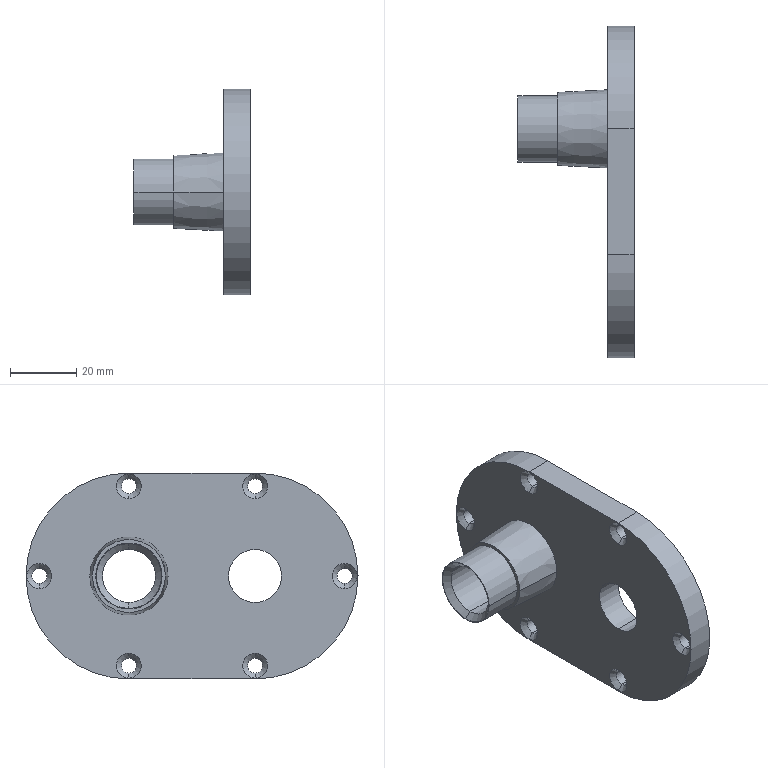Part | SolidWorks | features HoleWzd 3, Chamfer 1, Extrusion 1, Revolution 1 | 1 solid | 42 faces | box 35 x 100 x 62 mm | volume 43276 mm3 | cylinder 20 | cone 16 | plane 6 | commonest cylinder face diameters 4.5 x12 16 x4 20 x2 62 x2
STEP:
#1=CARTESIAN_POINT('',(1.5,-19.,24.75));
#2=VERTEX_POINT('',#1);
#3=CARTESIAN_POINT('',(1.5,-19.,29.25));
#4=VERTEX_POINT('',#3);
#5=CARTESIAN_POINT('',(1.5,-19.,27.));
#6=DIRECTION('',(-1.,0.,0.));
#7=DIRECTION('',(0.,0.,-1.));
#8=AXIS2_PLACEMENT_3D('',#5,#6,#7);
#9=CIRCLE('',#8,2.25);
#10=EDGE_CURVE('',#2,#4,#9,.T.);
#11=ORIENTED_EDGE('',*,*,#10,.F.);
#12=CARTESIAN_POINT('',(0.,-19.,23.25));
#13=VERTEX_POINT('',#12);
#14=CARTESIAN_POINT('',(1.5,-19.,24.75));
#15=DIRECTION('',(-0.7071,0.,-0.7071));
#16=VECTOR('',#15,1000.);
#17=LINE('',#14,#16);
#18=EDGE_CURVE('',#2,#13,#17,.T.);
#19=ORIENTED_EDGE('',*,*,#18,.T.);
#20=CARTESIAN_POINT('',(0.,-19.,30.75));
#21=VERTEX_POINT('',#20);
#22=CARTESIAN_POINT('',(0.,-19.,27.));
#23=DIRECTION('',(1.,0.,0.));
#24=DIRECTION('',(0.,0.,-1.));
#25=AXIS2_PLACEMENT_3D('',#22,#23,#24);
#26=CIRCLE('',#25,3.75);
#27=EDGE_CURVE('',#21,#13,#26,.T.);
#28=ORIENTED_EDGE('',*,*,#27,.F.);
#29=CARTESIAN_POINT('',(1.5,-19.,29.25));
#30=DIRECTION('',(-0.7071,0.,0.7071));
#31=VECTOR('',#30,1000.);
#32=LINE('',#29,#31);
#33=EDGE_CURVE('',#4,#21,#32,.T.);
#34=ORIENTED_EDGE('',*,*,#33,.F.);
#35=EDGE_LOOP('',(#11,#19,#28,#34));
#36=FACE_OUTER_BOUND('',#35,.T.);
#37=CARTESIAN_POINT('',(1.5,-19.,27.));
#38=DIRECTION('',(-1.,0.,0.));
#39=DIRECTION('',(0.,0.,1.));
#40=AXIS2_PLACEMENT_3D('',#37,#38,#39);
#41=CONICAL_SURFACE('',#40,2.25,0.7854);
#42=ADVANCED_FACE('',(#36),#41,.F.);
#43=CARTESIAN_POINT('',(1.5,-46.,-2.25));
#44=VERTEX_POINT('',#43);
#45=CARTESIAN_POINT('',(1.5,-46.,2.25));
#46=VERTEX_POINT('',#45);
#47=CARTESIAN_POINT('',(1.5,-46.,0.));
#48=DIRECTION('',(-1.,0.,0.));
#49=DIRECTION('',(0.,0.,-1.));
#50=AXIS2_PLACEMENT_3D('',#47,#48,#49);
#51=CIRCLE('',#50,2.25);
#52=EDGE_CURVE('',#44,#46,#51,.T.);
#53=ORIENTED_EDGE('',*,*,#52,.F.);
#54=CARTESIAN_POINT('',(0.,-46.,-3.75));
#55=VERTEX_POINT('',#54);
#56=CARTESIAN_POINT('',(1.5,-46.,-2.25));
#57=DIRECTION('',(-0.7071,0.,-0.7071));
#58=VECTOR('',#57,1000.);
#59=LINE('',#56,#58);
#60=EDGE_CURVE('',#44,#55,#59,.T.);
#61=ORIENTED_EDGE('',*,*,#60,.T.);
#62=CARTESIAN_POINT('',(0.,-46.,3.75));
#63=VERTEX_POINT('',#62);
#64=CARTESIAN_POINT('',(0.,-46.,0.));
#65=DIRECTION('',(1.,0.,0.));
#66=DIRECTION('',(0.,0.,-1.));
#67=AXIS2_PLACEMENT_3D('',#64,#65,#66);
#68=CIRCLE('',#67,3.75);
#69=EDGE_CURVE('',#63,#55,#68,.T.);
#70=ORIENTED_EDGE('',*,*,#69,.F.);
#71=CARTESIAN_POINT('',(1.5,-46.,2.25));
#72=DIRECTION('',(-0.7071,0.,0.7071));
#73=VECTOR('',#72,1000.);
#74=LINE('',#71,#73);
#75=EDGE_CURVE('',#46,#63,#74,.T.);
#76=ORIENTED_EDGE('',*,*,#75,.F.);
#77=EDGE_LOOP('',(#53,#61,#70,#76));
#78=FACE_OUTER_BOUND('',#77,.T.);
#79=CARTESIAN_POINT('',(1.5,-46.,0.));
#80=DIRECTION('',(-1.,0.,0.));
#81=DIRECTION('',(0.,0.,1.));
#82=AXIS2_PLACEMENT_3D('',#79,#80,#81);
#83=CONICAL_SURFACE('',#82,2.25,0.7854);
#84=ADVANCED_FACE('',(#78),#83,.F.);
#85=CARTESIAN_POINT('',(1.5,-19.,-29.25));
#86=VERTEX_POINT('',#85);
#87=CARTESIAN_POINT('',(1.5,-19.,-24.75));
#88=VERTEX_POINT('',#87);
#89=CARTESIAN_POINT('',(1.5,-19.,-27.));
#90=DIRECTION('',(-1.,0.,0.));
#91=DIRECTION('',(0.,0.,-1.));
#92=AXIS2_PLACEMENT_3D('',#89,#90,#91);
#93=CIRCLE('',#92,2.25);
#94=EDGE_CURVE('',#86,#88,#93,.T.);
#95=ORIENTED_EDGE('',*,*,#94,.F.);
#96=CARTESIAN_POINT('',(0.,-19.,-30.75));
#97=VERTEX_POINT('',#96);
#98=CARTESIAN_POINT('',(1.5,-19.,-29.25));
#99=DIRECTION('',(-0.7071,0.,-0.7071));
#100=VECTOR('',#99,1000.);
#101=LINE('',#98,#100);
#102=EDGE_CURVE('',#86,#97,#101,.T.);
#103=ORIENTED_EDGE('',*,*,#102,.T.);
#104=CARTESIAN_POINT('',(0.,-19.,-23.25));
#105=VERTEX_POINT('',#104);
#106=CARTESIAN_POINT('',(0.,-19.,-27.));
#107=DIRECTION('',(1.,0.,0.));
#108=DIRECTION('',(0.,0.,-1.));
#109=AXIS2_PLACEMENT_3D('',#106,#107,#108);
#110=CIRCLE('',#109,3.75);
#111=EDGE_CURVE('',#105,#97,#110,.T.);
#112=ORIENTED_EDGE('',*,*,#111,.F.);
#113=CARTESIAN_POINT('',(1.5,-19.,-24.75));
#114=DIRECTION('',(-0.7071,0.,0.7071));
#115=VECTOR('',#114,1000.);
#116=LINE('',#113,#115);
#117=EDGE_CURVE('',#88,#105,#116,.T.);
#118=ORIENTED_EDGE('',*,*,#117,.F.);
#119=EDGE_LOOP('',(#95,#103,#112,#118));
#120=FACE_OUTER_BOUND('',#119,.T.);
#121=CARTESIAN_POINT('',(1.5,-19.,-27.));
#122=DIRECTION('',(-1.,0.,0.));
#123=DIRECTION('',(0.,0.,1.));
#124=AXIS2_PLACEMENT_3D('',#121,#122,#123);
#125=CONICAL_SURFACE('',#124,2.25,0.7854);
#126=ADVANCED_FACE('',(#120),#125,.F.);
#127=CARTESIAN_POINT('',(1.5,19.,-29.25));
#128=VERTEX_POINT('',#127);
#129=CARTESIAN_POINT('',(1.5,19.,-24.75));
#130=VERTEX_POINT('',#129);
#131=CARTESIAN_POINT('',(1.5,19.,-27.));
#132=DIRECTION('',(-1.,0.,0.));
#133=DIRECTION('',(0.,0.,-1.));
#134=AXIS2_PLACEMENT_3D('',#131,#132,#133);
#135=CIRCLE('',#134,2.25);
#136=EDGE_CURVE('',#128,#130,#135,.T.);
#137=ORIENTED_EDGE('',*,*,#136,.F.);
#138=CARTESIAN_POINT('',(0.,19.,-30.75));
#139=VERTEX_POINT('',#138);
#140=CARTESIAN_POINT('',(1.5,19.,-29.25));
#141=DIRECTION('',(-0.7071,0.,-0.7071));
#142=VECTOR('',#141,1000.);
#143=LINE('',#140,#142);
#144=EDGE_CURVE('',#128,#139,#143,.T.);
#145=ORIENTED_EDGE('',*,*,#144,.T.);
#146=CARTESIAN_POINT('',(0.,19.,-23.25));
#147=VERTEX_POINT('',#146);
#148=CARTESIAN_POINT('',(0.,19.,-27.));
#149=DIRECTION('',(1.,0.,0.));
#150=DIRECTION('',(0.,0.,-1.));
#151=AXIS2_PLACEMENT_3D('',#148,#149,#150);
#152=CIRCLE('',#151,3.75);
#153=EDGE_CURVE('',#147,#139,#152,.T.);
#154=ORIENTED_EDGE('',*,*,#153,.F.);
#155=CARTESIAN_POINT('',(1.5,19.,-24.75));
#156=DIRECTION('',(-0.7071,0.,0.7071));
#157=VECTOR('',#156,1000.);
#158=LINE('',#155,#157);
#159=EDGE_CURVE('',#130,#147,#158,.T.);
#160=ORIENTED_EDGE('',*,*,#159,.F.);
#161=EDGE_LOOP('',(#137,#145,#154,#160));
#162=FACE_OUTER_BOUND('',#161,.T.);
#163=CARTESIAN_POINT('',(1.5,19.,-27.));
#164=DIRECTION('',(-1.,0.,0.));
#165=DIRECTION('',(0.,0.,1.));
#166=AXIS2_PLACEMENT_3D('',#163,#164,#165);
#167=CONICAL_SURFACE('',#166,2.25,0.7854);
#168=ADVANCED_FACE('',(#162),#167,.F.);
#169=CARTESIAN_POINT('',(1.5,46.,-2.25));
#170=VERTEX_POINT('',#169);
#171=CARTESIAN_POINT('',(1.5,46.,2.25));
#172=VERTEX_POINT('',#171);
#173=CARTESIAN_POINT('',(1.5,46.,0.));
#174=DIRECTION('',(-1.,0.,0.));
#175=DIRECTION('',(0.,0.,-1.));
#176=AXIS2_PLACEMENT_3D('',#173,#174,#175);
#177=CIRCLE('',#176,2.25);
#178=EDGE_CURVE('',#170,#172,#177,.T.);
#179=ORIENTED_EDGE('',*,*,#178,.F.);
#180=CARTESIAN_POINT('',(0.,46.,-3.75));
#181=VERTEX_POINT('',#180);
#182=CARTESIAN_POINT('',(1.5,46.,-2.25));
#183=DIRECTION('',(-0.7071,0.,-0.7071));
#184=VECTOR('',#183,1000.);
#185=LINE('',#182,#184);
#186=EDGE_CURVE('',#170,#181,#185,.T.);
#187=ORIENTED_EDGE('',*,*,#186,.T.);
#188=CARTESIAN_POINT('',(0.,46.,3.75));
#189=VERTEX_POINT('',#188);
#190=CARTESIAN_POINT('',(0.,46.,0.));
#191=DIRECTION('',(1.,0.,0.));
#192=DIRECTION('',(0.,0.,-1.));
#193=AXIS2_PLACEMENT_3D('',#190,#191,#192);
#194=CIRCLE('',#193,3.75);
#195=EDGE_CURVE('',#189,#181,#194,.T.);
#196=ORIENTED_EDGE('',*,*,#195,.F.);
#197=CARTESIAN_POINT('',(1.5,46.,2.25));
#198=DIRECTION('',(-0.7071,0.,0.7071));
#199=VECTOR('',#198,1000.);
#200=LINE('',#197,#199);
#201=EDGE_CURVE('',#172,#189,#200,.T.);
#202=ORIENTED_EDGE('',*,*,#201,.F.);
#203=EDGE_LOOP('',(#179,#187,#196,#202));
#204=FACE_OUTER_BOUND('',#203,.T.);
#205=CARTESIAN_POINT('',(1.5,46.,0.));
#206=DIRECTION('',(-1.,0.,0.));
#207=DIRECTION('',(0.,0.,1.));
#208=AXIS2_PLACEMENT_3D('',#205,#206,#207);
#209=CONICAL_SURFACE('',#208,2.25,0.7854);
#210=ADVANCED_FACE('',(#204),#209,.F.);
#211=CARTESIAN_POINT('',(1.5,19.,24.75));
#212=VERTEX_POINT('',#211);
#213=CARTESIAN_POINT('',(1.5,19.,29.25));
#214=VERTEX_POINT('',#213);
#215=CARTESIAN_POINT('',(1.5,19.,27.));
#216=DIRECTION('',(-1.,0.,0.));
#217=DIRECTION('',(0.,0.,-1.));
#218=AXIS2_PLACEMENT_3D('',#215,#216,#217);
#219=CIRCLE('',#218,2.25);
#220=EDGE_CURVE('',#212,#214,#219,.T.);
#221=ORIENTED_EDGE('',*,*,#220,.F.);
#222=CARTESIAN_POINT('',(0.,19.,23.25));
#223=VERTEX_POINT('',#222);
#224=CARTESIAN_POINT('',(1.5,19.,24.75));
#225=DIRECTION('',(-0.7071,0.,-0.7071));
#226=VECTOR('',#225,1000.);
#227=LINE('',#224,#226);
#228=EDGE_CURVE('',#212,#223,#227,.T.);
#229=ORIENTED_EDGE('',*,*,#228,.T.);
#230=CARTESIAN_POINT('',(0.,19.,30.75));
#231=VERTEX_POINT('',#230);
#232=CARTESIAN_POINT('',(0.,19.,27.));
#233=DIRECTION('',(1.,0.,0.));
#234=DIRECTION('',(0.,0.,-1.));
#235=AXIS2_PLACEMENT_3D('',#232,#233,#234);
#236=CIRCLE('',#235,3.75);
#237=EDGE_CURVE('',#231,#223,#236,.T.);
#238=ORIENTED_EDGE('',*,*,#237,.F.);
#239=CARTESIAN_POINT('',(1.5,19.,29.25));
#240=DIRECTION('',(-0.7071,0.,0.7071));
#241=VECTOR('',#240,1000.);
#242=LINE('',#239,#241);
#243=EDGE_CURVE('',#214,#231,#242,.T.);
#244=ORIENTED_EDGE('',*,*,#243,.F.);
#245=EDGE_LOOP('',(#221,#229,#238,#244));
#246=FACE_OUTER_BOUND('',#245,.T.);
#247=CARTESIAN_POINT('',(1.5,19.,27.));
#248=DIRECTION('',(-1.,0.,0.));
#249=DIRECTION('',(0.,0.,1.));
#250=AXIS2_PLACEMENT_3D('',#247,#248,#249);
#251=CONICAL_SURFACE('',#250,2.25,0.7854);
#252=ADVANCED_FACE('',(#246),#251,.F.);
#253=CARTESIAN_POINT('',(8.,46.,-2.25));
#254=VERTEX_POINT('',#253);
#255=CARTESIAN_POINT('',(8.,46.,2.25));
#256=VERTEX_POINT('',#255);
#257=CARTESIAN_POINT('',(8.,46.,0.));
#258=DIRECTION('',(-1.,0.,0.));
#259=DIRECTION('',(0.,0.,1.));
#260=AXIS2_PLACEMENT_3D('',#257,#258,#259);
#261=CIRCLE('',#260,2.25);
#262=EDGE_CURVE('',#254,#256,#261,.T.);
#263=ORIENTED_EDGE('',*,*,#262,.F.);
#264=CARTESIAN_POINT('',(0.,46.,-2.25));
#265=DIRECTION('',(-1.,0.,0.));
#266=VECTOR('',#265,1000.);
#267=LINE('',#264,#266);
#268=EDGE_CURVE('',#254,#170,#267,.T.);
#269=ORIENTED_EDGE('',*,*,#268,.T.);
#270=ORIENTED_EDGE('',*,*,#178,.T.);
#271=CARTESIAN_POINT('',(0.,46.,2.25));
#272=DIRECTION('',(-1.,0.,0.));
#273=VECTOR('',#272,1000.);
#274=LINE('',#271,#273);
#275=EDGE_CURVE('',#256,#172,#274,.T.);
#276=ORIENTED_EDGE('',*,*,#275,.F.);
#277=EDGE_LOOP('',(#263,#269,#270,#276));
#278=FACE_OUTER_BOUND('',#277,.T.);
#279=CARTESIAN_POINT('',(0.,46.,0.));
#280=DIRECTION('',(-1.,0.,0.));
#281=DIRECTION('',(0.,0.,1.));
#282=AXIS2_PLACEMENT_3D('',#279,#280,#281);
#283=CYLINDRICAL_SURFACE('',#282,2.25);
#284=ADVANCED_FACE('',(#278),#283,.F.);
#285=CARTESIAN_POINT('',(8.,19.,24.75));
#286=VERTEX_POINT('',#285);
#287=CARTESIAN_POINT('',(8.,19.,29.25));
#288=VERTEX_POINT('',#287);
#289=CARTESIAN_POINT('',(8.,19.,27.));
#290=DIRECTION('',(-1.,0.,0.));
#291=DIRECTION('',(0.,0.,1.));
#292=AXIS2_PLACEMENT_3D('',#289,#290,#291);
#293=CIRCLE('',#292,2.25);
#294=EDGE_CURVE('',#286,#288,#293,.T.);
#295=ORIENTED_EDGE('',*,*,#294,.F.);
#296=CARTESIAN_POINT('',(0.,19.,24.75));
#297=DIRECTION('',(-1.,0.,0.));
#298=VECTOR('',#297,1000.);
#299=LINE('',#296,#298);
#300=EDGE_CURVE('',#286,#212,#299,.T.);
#301=ORIENTED_EDGE('',*,*,#300,.T.);
#302=ORIENTED_EDGE('',*,*,#220,.T.);
#303=CARTESIAN_POINT('',(0.,19.,29.25));
#304=DIRECTION('',(-1.,0.,0.));
#305=VECTOR('',#304,1000.);
#306=LINE('',#303,#305);
#307=EDGE_CURVE('',#288,#214,#306,.T.);
#308=ORIENTED_EDGE('',*,*,#307,.F.);
#309=EDGE_LOOP('',(#295,#301,#302,#308));
#310=FACE_OUTER_BOUND('',#309,.T.);
#311=CARTESIAN_POINT('',(0.,19.,27.));
#312=DIRECTION('',(-1.,0.,0.));
#313=DIRECTION('',(0.,0.,1.));
#314=AXIS2_PLACEMENT_3D('',#311,#312,#313);
#315=CYLINDRICAL_SURFACE('',#314,2.25);
#316=ADVANCED_FACE('',(#310),#315,.F.);
#317=CARTESIAN_POINT('',(8.,19.,-29.25));
#318=VERTEX_POINT('',#317);
#319=CARTESIAN_POINT('',(8.,19.,-24.75));
#320=VERTEX_POINT('',#319);
#321=CARTESIAN_POINT('',(8.,19.,-27.));
#322=DIRECTION('',(-1.,0.,0.));
#323=DIRECTION('',(0.,0.,1.));
#324=AXIS2_PLACEMENT_3D('',#321,#322,#323);
#325=CIRCLE('',#324,2.25);
#326=EDGE_CURVE('',#318,#320,#325,.T.);
#327=ORIENTED_EDGE('',*,*,#326,.F.);
#328=CARTESIAN_POINT('',(0.,19.,-29.25));
#329=DIRECTION('',(-1.,0.,0.));
#330=VECTOR('',#329,1000.);
#331=LINE('',#328,#330);
#332=EDGE_CURVE('',#318,#128,#331,.T.);
#333=ORIENTED_EDGE('',*,*,#332,.T.);
#334=ORIENTED_EDGE('',*,*,#136,.T.);
#335=CARTESIAN_POINT('',(0.,19.,-24.75));
#336=DIRECTION('',(-1.,0.,0.));
#337=VECTOR('',#336,1000.);
#338=LINE('',#335,#337);
#339=EDGE_CURVE('',#320,#130,#338,.T.);
#340=ORIENTED_EDGE('',*,*,#339,.F.);
#341=EDGE_LOOP('',(#327,#333,#334,#340));
#342=FACE_OUTER_BOUND('',#341,.T.);
#343=CARTESIAN_POINT('',(0.,19.,-27.));
#344=DIRECTION('',(-1.,0.,0.));
#345=DIRECTION('',(0.,0.,1.));
#346=AXIS2_PLACEMENT_3D('',#343,#344,#345);
#347=CYLINDRICAL_SURFACE('',#346,2.25);
#348=ADVANCED_FACE('',(#342),#347,.F.);
#349=CARTESIAN_POINT('',(8.,-19.,24.75));
#350=VERTEX_POINT('',#349);
#351=CARTESIAN_POINT('',(8.,-19.,29.25));
#352=VERTEX_POINT('',#351);
#353=CARTESIAN_POINT('',(8.,-19.,27.));
#354=DIRECTION('',(-1.,0.,0.));
#355=DIRECTION('',(0.,0.,1.));
#356=AXIS2_PLACEMENT_3D('',#353,#354,#355);
#357=CIRCLE('',#356,2.25);
#358=EDGE_CURVE('',#350,#352,#357,.T.);
#359=ORIENTED_EDGE('',*,*,#358,.F.);
#360=CARTESIAN_POINT('',(0.,-19.,24.75));
#361=DIRECTION('',(-1.,0.,0.));
#362=VECTOR('',#361,1000.);
#363=LINE('',#360,#362);
#364=EDGE_CURVE('',#350,#2,#363,.T.);
#365=ORIENTED_EDGE('',*,*,#364,.T.);
#366=ORIENTED_EDGE('',*,*,#10,.T.);
#367=CARTESIAN_POINT('',(0.,-19.,29.25));
#368=DIRECTION('',(-1.,0.,0.));
#369=VECTOR('',#368,1000.);
#370=LINE('',#367,#369);
#371=EDGE_CURVE('',#352,#4,#370,.T.);
#372=ORIENTED_EDGE('',*,*,#371,.F.);
#373=EDGE_LOOP('',(#359,#365,#366,#372));
#374=FACE_OUTER_BOUND('',#373,.T.);
#375=CARTESIAN_POINT('',(0.,-19.,27.));
#376=DIRECTION('',(-1.,0.,0.));
#377=DIRECTION('',(0.,0.,1.));
#378=AXIS2_PLACEMENT_3D('',#375,#376,#377);
#379=CYLINDRICAL_SURFACE('',#378,2.25);
#380=ADVANCED_FACE('',(#374),#379,.F.);
#381=CARTESIAN_POINT('',(8.,-19.,-29.25));
#382=VERTEX_POINT('',#381);
#383=CARTESIAN_POINT('',(8.,-19.,-24.75));
#384=VERTEX_POINT('',#383);
#385=CARTESIAN_POINT('',(8.,-19.,-27.));
#386=DIRECTION('',(-1.,0.,0.));
#387=DIRECTION('',(0.,0.,1.));
#388=AXIS2_PLACEMENT_3D('',#385,#386,#387);
#389=CIRCLE('',#388,2.25);
#390=EDGE_CURVE('',#382,#384,#389,.T.);
#391=ORIENTED_EDGE('',*,*,#390,.F.);
#392=CARTESIAN_POINT('',(0.,-19.,-29.25));
#393=DIRECTION('',(-1.,0.,0.));
#394=VECTOR('',#393,1000.);
#395=LINE('',#392,#394);
#396=EDGE_CURVE('',#382,#86,#395,.T.);
#397=ORIENTED_EDGE('',*,*,#396,.T.);
#398=ORIENTED_EDGE('',*,*,#94,.T.);
#399=CARTESIAN_POINT('',(0.,-19.,-24.75));
#400=DIRECTION('',(-1.,0.,0.));
#401=VECTOR('',#400,1000.);
#402=LINE('',#399,#401);
#403=EDGE_CURVE('',#384,#88,#402,.T.);
#404=ORIENTED_EDGE('',*,*,#403,.F.);
#405=EDGE_LOOP('',(#391,#397,#398,#404));
#406=FACE_OUTER_BOUND('',#405,.T.);
#407=CARTESIAN_POINT('',(0.,-19.,-27.));
#408=DIRECTION('',(-1.,0.,0.));
#409=DIRECTION('',(0.,0.,1.));
#410=AXIS2_PLACEMENT_3D('',#407,#408,#409);
#411=CYLINDRICAL_SURFACE('',#410,2.25);
#412=ADVANCED_FACE('',(#406),#411,.F.);
#413=CARTESIAN_POINT('',(8.,-46.,-2.25));
#414=VERTEX_POINT('',#413);
#415=CARTESIAN_POINT('',(8.,-46.,2.25));
#416=VERTEX_POINT('',#415);
#417=CARTESIAN_POINT('',(8.,-46.,0.));
#418=DIRECTION('',(-1.,0.,0.));
#419=DIRECTION('',(0.,0.,1.));
#420=AXIS2_PLACEMENT_3D('',#417,#418,#419);
#421=CIRCLE('',#420,2.25);
#422=EDGE_CURVE('',#414,#416,#421,.T.);
#423=ORIENTED_EDGE('',*,*,#422,.F.);
#424=CARTESIAN_POINT('',(0.,-46.,-2.25));
#425=DIRECTION('',(-1.,0.,0.));
#426=VECTOR('',#425,1000.);
#427=LINE('',#424,#426);
#428=EDGE_CURVE('',#414,#44,#427,.T.);
#429=ORIENTED_EDGE('',*,*,#428,.T.);
#430=ORIENTED_EDGE('',*,*,#52,.T.);
#431=CARTESIAN_POINT('',(0.,-46.,2.25));
#432=DIRECTION('',(-1.,0.,0.));
#433=VECTOR('',#432,1000.);
#434=LINE('',#431,#433);
#435=EDGE_CURVE('',#416,#46,#434,.T.);
#436=ORIENTED_EDGE('',*,*,#435,.F.);
#437=EDGE_LOOP('',(#423,#429,#430,#436));
#438=FACE_OUTER_BOUND('',#437,.T.);
#439=CARTESIAN_POINT('',(0.,-46.,0.));
#440=DIRECTION('',(-1.,0.,0.));
#441=DIRECTION('',(0.,0.,1.));
#442=AXIS2_PLACEMENT_3D('',#439,#440,#441);
#443=CYLINDRICAL_SURFACE('',#442,2.25);
#444=ADVANCED_FACE('',(#438),#443,.F.);
#445=CARTESIAN_POINT('',(-25.2,19.,-8.));
#446=VERTEX_POINT('',#445);
#447=CARTESIAN_POINT('',(-25.2,19.,8.));
#448=VERTEX_POINT('',#447);
#449=CARTESIAN_POINT('',(-25.2,19.,0.));
#450=DIRECTION('',(-1.,0.,0.));
#451=DIRECTION('',(0.,0.,1.));
#452=AXIS2_PLACEMENT_3D('',#449,#450,#451);
#453=CIRCLE('',#452,8.);
#454=EDGE_CURVE('',#446,#448,#453,.T.);
#455=ORIENTED_EDGE('',*,*,#454,.F.);
#456=CARTESIAN_POINT('',(-27.,19.,-9.8));
#457=VERTEX_POINT('',#456);
#458=CARTESIAN_POINT('',(-27.,19.,-9.8));
#459=DIRECTION('',(-0.7071,0.,-0.7071));
#460=VECTOR('',#459,1000.);
#461=LINE('',#458,#460);
#462=EDGE_CURVE('',#446,#457,#461,.T.);
#463=ORIENTED_EDGE('',*,*,#462,.T.);
#464=CARTESIAN_POINT('',(-27.,19.,9.8));
#465=VERTEX_POINT('',#464);
#466=CARTESIAN_POINT('',(-27.,19.,0.));
#467=DIRECTION('',(-1.,0.,0.));
#468=DIRECTION('',(0.,0.,1.));
#469=AXIS2_PLACEMENT_3D('',#466,#467,#468);
#470=CIRCLE('',#469,9.8);
#471=EDGE_CURVE('',#457,#465,#470,.T.);
#472=ORIENTED_EDGE('',*,*,#471,.T.);
#473=CARTESIAN_POINT('',(-27.,19.,9.8));
#474=DIRECTION('',(-0.7071,0.,0.7071));
#475=VECTOR('',#474,1000.);
#476=LINE('',#473,#475);
#477=EDGE_CURVE('',#448,#465,#476,.T.);
#478=ORIENTED_EDGE('',*,*,#477,.F.);
#479=EDGE_LOOP('',(#455,#463,#472,#478));
#480=FACE_OUTER_BOUND('',#479,.T.);
#481=CARTESIAN_POINT('',(-27.,19.,0.));
#482=DIRECTION('',(-1.,0.,0.));
#483=DIRECTION('',(0.,0.,1.));
#484=AXIS2_PLACEMENT_3D('',#481,#482,#483);
#485=CONICAL_SURFACE('',#484,9.8,0.7854);
#486=ADVANCED_FACE('',(#480),#485,.F.);
#487=CARTESIAN_POINT('',(8.,19.,-8.));
#488=VERTEX_POINT('',#487);
#489=CARTESIAN_POINT('',(8.,19.,8.));
#490=VERTEX_POINT('',#489);
#491=CARTESIAN_POINT('',(8.,19.,0.));
#492=DIRECTION('',(-1.,0.,0.));
#493=DIRECTION('',(0.,0.,1.));
#494=AXIS2_PLACEMENT_3D('',#491,#492,#493);
#495=CIRCLE('',#494,8.);
#496=EDGE_CURVE('',#488,#490,#495,.T.);
#497=ORIENTED_EDGE('',*,*,#496,.F.);
#498=CARTESIAN_POINT('',(-27.,19.,-8.));
#499=DIRECTION('',(-1.,0.,0.));
#500=VECTOR('',#499,1000.);
#501=LINE('',#498,#500);
#502=EDGE_CURVE('',#488,#446,#501,.T.);
#503=ORIENTED_EDGE('',*,*,#502,.T.);
#504=ORIENTED_EDGE('',*,*,#454,.T.);
#505=CARTESIAN_POINT('',(-27.,19.,8.));
#506=DIRECTION('',(-1.,0.,0.));
#507=VECTOR('',#506,1000.);
#508=LINE('',#505,#507);
#509=EDGE_CURVE('',#490,#448,#508,.T.);
#510=ORIENTED_EDGE('',*,*,#509,.F.);
#511=EDGE_LOOP('',(#497,#503,#504,#510));
#512=FACE_OUTER_BOUND('',#511,.T.);
#513=CARTESIAN_POINT('',(-27.,19.,0.));
#514=DIRECTION('',(-1.,0.,0.));
#515=DIRECTION('',(0.,0.,1.));
#516=AXIS2_PLACEMENT_3D('',#513,#514,#515);
#517=CYLINDRICAL_SURFACE('',#516,8.);
#518=ADVANCED_FACE('',(#512),#517,.F.);
#519=CARTESIAN_POINT('',(8.,-19.,-8.));
#520=VERTEX_POINT('',#519);
#521=CARTESIAN_POINT('',(8.,-19.,8.));
#522=VERTEX_POINT('',#521);
#523=CARTESIAN_POINT('',(8.,-19.,0.));
#524=DIRECTION('',(-1.,0.,0.));
#525=DIRECTION('',(0.,0.,1.));
#526=AXIS2_PLACEMENT_3D('',#523,#524,#525);
#527=CIRCLE('',#526,8.);
#528=EDGE_CURVE('',#520,#522,#527,.T.);
#529=ORIENTED_EDGE('',*,*,#528,.F.);
#530=CARTESIAN_POINT('',(0.,-19.,-8.));
#531=VERTEX_POINT('',#530);
#532=CARTESIAN_POINT('',(0.,-19.,-8.));
#533=DIRECTION('',(-1.,0.,0.));
#534=VECTOR('',#533,1000.);
#535=LINE('',#532,#534);
#536=EDGE_CURVE('',#520,#531,#535,.T.);
#537=ORIENTED_EDGE('',*,*,#536,.T.);
#538=CARTESIAN_POINT('',(0.,-19.,8.));
#539=VERTEX_POINT('',#538);
#540=CARTESIAN_POINT('',(0.,-19.,0.));
#541=DIRECTION('',(-1.,0.,0.));
#542=DIRECTION('',(0.,0.,1.));
#543=AXIS2_PLACEMENT_3D('',#540,#541,#542);
#544=CIRCLE('',#543,8.);
#545=EDGE_CURVE('',#531,#539,#544,.T.);
#546=ORIENTED_EDGE('',*,*,#545,.T.);
#547=CARTESIAN_POINT('',(0.,-19.,8.));
#548=DIRECTION('',(-1.,0.,0.));
#549=VECTOR('',#548,1000.);
#550=LINE('',#547,#549);
#551=EDGE_CURVE('',#522,#539,#550,.T.);
#552=ORIENTED_EDGE('',*,*,#551,.F.);
#553=EDGE_LOOP('',(#529,#537,#546,#552));
#554=FACE_OUTER_BOUND('',#553,.T.);
#555=CARTESIAN_POINT('',(0.,-19.,0.));
#556=DIRECTION('',(-1.,0.,0.));
#557=DIRECTION('',(0.,0.,1.));
#558=AXIS2_PLACEMENT_3D('',#555,#556,#557);
#559=CYLINDRICAL_SURFACE('',#558,8.);
#560=ADVANCED_FACE('',(#554),#559,.F.);
#561=CARTESIAN_POINT('',(-15.,30.,0.));
#562=VERTEX_POINT('',#561);
#563=CARTESIAN_POINT('',(-15.,8.,0.));
#564=VERTEX_POINT('',#563);
#565=CARTESIAN_POINT('',(-15.,19.,0.));
#566=DIRECTION('',(1.,0.,0.));
#567=DIRECTION('',(0.,1.,0.));
#568=AXIS2_PLACEMENT_3D('',#565,#566,#567);
#569=CIRCLE('',#568,11.);
#570=EDGE_CURVE('',#562,#564,#569,.T.);
#571=ORIENTED_EDGE('',*,*,#570,.T.);
#572=CARTESIAN_POINT('',(0.,7.214,0.));
#573=VERTEX_POINT('',#572);
#574=CARTESIAN_POINT('',(0.,7.214,0.));
#575=DIRECTION('',(0.9986,-0.05234,0.));
#576=VECTOR('',#575,1000.);
#577=LINE('',#574,#576);
#578=EDGE_CURVE('',#564,#573,#577,.T.);
#579=ORIENTED_EDGE('',*,*,#578,.T.);
#580=CARTESIAN_POINT('',(0.,30.786,0.));
#581=VERTEX_POINT('',#580);
#582=CARTESIAN_POINT('',(0.,19.,0.));
#583=DIRECTION('',(1.,0.,0.));
#584=DIRECTION('',(0.,1.,0.));
#585=AXIS2_PLACEMENT_3D('',#582,#583,#584);
#586=CIRCLE('',#585,11.786);
#587=EDGE_CURVE('',#581,#573,#586,.T.);
#588=ORIENTED_EDGE('',*,*,#587,.F.);
#589=CARTESIAN_POINT('',(0.,30.786,0.));
#590=DIRECTION('',(0.9986,0.05234,0.));
#591=VECTOR('',#590,1000.);
#592=LINE('',#589,#591);
#593=EDGE_CURVE('',#562,#581,#592,.T.);
#594=ORIENTED_EDGE('',*,*,#593,.F.);
#595=EDGE_LOOP('',(#571,#579,#588,#594));
#596=FACE_OUTER_BOUND('',#595,.T.);
#597=CARTESIAN_POINT('',(0.,19.,0.));
#598=DIRECTION('',(1.,0.,0.));
#599=DIRECTION('',(0.,1.,0.));
#600=AXIS2_PLACEMENT_3D('',#597,#598,#599);
#601=CONICAL_SURFACE('',#600,11.786,0.05236);
#602=ADVANCED_FACE('',(#596),#601,.T.);
#603=CARTESIAN_POINT('',(-27.,29.,0.));
#604=VERTEX_POINT('',#603);
#605=CARTESIAN_POINT('',(-27.,9.,0.));
#606=VERTEX_POINT('',#605);
#607=CARTESIAN_POINT('',(-27.,19.,0.));
#608=DIRECTION('',(1.,0.,0.));
#609=DIRECTION('',(0.,1.,0.));
#610=AXIS2_PLACEMENT_3D('',#607,#608,#609);
#611=CIRCLE('',#610,10.);
#612=EDGE_CURVE('',#604,#606,#611,.T.);
#613=ORIENTED_EDGE('',*,*,#612,.T.);
#614=CARTESIAN_POINT('',(-15.,9.,0.));
#615=VERTEX_POINT('',#614);
#616=CARTESIAN_POINT('',(-27.,9.,0.));
#617=DIRECTION('',(1.,0.,0.));
#618=VECTOR('',#617,1000.);
#619=LINE('',#616,#618);
#620=EDGE_CURVE('',#606,#615,#619,.T.);
#621=ORIENTED_EDGE('',*,*,#620,.T.);
#622=CARTESIAN_POINT('',(-15.,29.,0.));
#623=VERTEX_POINT('',#622);
#624=CARTESIAN_POINT('',(-15.,19.,0.));
#625=DIRECTION('',(1.,0.,0.));
#626=DIRECTION('',(0.,1.,0.));
#627=AXIS2_PLACEMENT_3D('',#624,#625,#626);
#628=CIRCLE('',#627,10.);
#629=EDGE_CURVE('',#623,#615,#628,.T.);
#630=ORIENTED_EDGE('',*,*,#629,.F.);
#631=CARTESIAN_POINT('',(-27.,29.,0.));
#632=DIRECTION('',(1.,0.,0.));
#633=VECTOR('',#632,1000.);
#634=LINE('',#631,#633);
#635=EDGE_CURVE('',#604,#623,#634,.T.);
#636=ORIENTED_EDGE('',*,*,#635,.F.);
#637=EDGE_LOOP('',(#613,#621,#630,#636));
#638=FACE_OUTER_BOUND('',#637,.T.);
#639=CARTESIAN_POINT('',(-27.,19.,0.));
#640=DIRECTION('',(1.,0.,0.));
#641=DIRECTION('',(0.,1.,0.));
#642=AXIS2_PLACEMENT_3D('',#639,#640,#641);
#643=CYLINDRICAL_SURFACE('',#642,10.);
#644=ADVANCED_FACE('',(#638),#643,.T.);
#645=CARTESIAN_POINT('',(8.,-19.,31.));
#646=VERTEX_POINT('',#645);
#647=CARTESIAN_POINT('',(8.,-19.,-31.));
#648=VERTEX_POINT('',#647);
#649=CARTESIAN_POINT('',(8.,-19.,0.));
#650=DIRECTION('',(1.,0.,0.));
#651=DIRECTION('',(0.,0.,-1.));
#652=AXIS2_PLACEMENT_3D('',#649,#650,#651);
#653=CIRCLE('',#652,31.);
#654=EDGE_CURVE('',#646,#648,#653,.T.);
#655=ORIENTED_EDGE('',*,*,#654,.F.);
#656=CARTESIAN_POINT('',(0.,-19.,31.));
#657=VERTEX_POINT('',#656);
#658=CARTESIAN_POINT('',(0.,-19.,31.));
#659=DIRECTION('',(1.,0.,0.));
#660=VECTOR('',#659,1000.);
#661=LINE('',#658,#660);
#662=EDGE_CURVE('',#657,#646,#661,.T.);
#663=ORIENTED_EDGE('',*,*,#662,.F.);
#664=CARTESIAN_POINT('',(0.,-19.,-31.));
#665=VERTEX_POINT('',#664);
#666=CARTESIAN_POINT('',(0.,-19.,0.));
#667=DIRECTION('',(1.,0.,0.));
#668=DIRECTION('',(0.,0.,-1.));
#669=AXIS2_PLACEMENT_3D('',#666,#667,#668);
#670=CIRCLE('',#669,31.);
#671=EDGE_CURVE('',#657,#665,#670,.T.);
#672=ORIENTED_EDGE('',*,*,#671,.T.);
#673=CARTESIAN_POINT('',(0.,-19.,-31.));
#674=DIRECTION('',(1.,0.,0.));
#675=VECTOR('',#674,1000.);
#676=LINE('',#673,#675);
#677=EDGE_CURVE('',#665,#648,#676,.T.);
#678=ORIENTED_EDGE('',*,*,#677,.T.);
#679=EDGE_LOOP('',(#655,#663,#672,#678));
#680=FACE_OUTER_BOUND('',#679,.T.);
#681=CARTESIAN_POINT('',(0.,-19.,0.));
#682=DIRECTION('',(1.,0.,0.));
#683=DIRECTION('',(0.,0.,-1.));
#684=AXIS2_PLACEMENT_3D('',#681,#682,#683);
#685=CYLINDRICAL_SURFACE('',#684,31.);
#686=ADVANCED_FACE('',(#680),#685,.T.);
#687=CARTESIAN_POINT('',(8.,19.,31.));
#688=VERTEX_POINT('',#687);
#689=CARTESIAN_POINT('',(8.,19.,31.));
#690=DIRECTION('',(0.,-1.,0.));
#691=VECTOR('',#690,1000.);
#692=LINE('',#689,#691);
#693=EDGE_CURVE('',#688,#646,#692,.T.);
#694=ORIENTED_EDGE('',*,*,#693,.F.);
#695=CARTESIAN_POINT('',(0.,19.,31.));
#696=VERTEX_POINT('',#695);
#697=CARTESIAN_POINT('',(0.,19.,31.));
#698=DIRECTION('',(1.,0.,0.));
#699=VECTOR('',#698,1000.);
#700=LINE('',#697,#699);
#701=EDGE_CURVE('',#696,#688,#700,.T.);
#702=ORIENTED_EDGE('',*,*,#701,.F.);
#703=CARTESIAN_POINT('',(0.,19.,31.));
#704=DIRECTION('',(0.,-1.,0.));
#705=VECTOR('',#704,1000.);
#706=LINE('',#703,#705);
#707=EDGE_CURVE('',#696,#657,#706,.T.);
#708=ORIENTED_EDGE('',*,*,#707,.T.);
#709=ORIENTED_EDGE('',*,*,#662,.T.);
#710=EDGE_LOOP('',(#694,#702,#708,#709));
#711=FACE_OUTER_BOUND('',#710,.T.);
#712=CARTESIAN_POINT('',(0.,19.,31.));
#713=DIRECTION('',(0.,0.,1.));
#714=DIRECTION('',(1.,0.,0.));
#715=AXIS2_PLACEMENT_3D('',#712,#713,#714);
#716=PLANE('',#715);
#717=ADVANCED_FACE('',(#711),#716,.T.);
#718=CARTESIAN_POINT('',(8.,19.,-31.));
#719=VERTEX_POINT('',#718);
#720=CARTESIAN_POINT('',(8.,19.,0.));
#721=DIRECTION('',(1.,0.,0.));
#722=DIRECTION('',(0.,0.,-1.));
#723=AXIS2_PLACEMENT_3D('',#720,#721,#722);
#724=CIRCLE('',#723,31.);
#725=EDGE_CURVE('',#719,#688,#724,.T.);
#726=ORIENTED_EDGE('',*,*,#725,.F.);
#727=CARTESIAN_POINT('',(0.,19.,-31.));
#728=VERTEX_POINT('',#727);
#729=CARTESIAN_POINT('',(0.,19.,-31.));
#730=DIRECTION('',(1.,0.,0.));
#731=VECTOR('',#730,1000.);
#732=LINE('',#729,#731);
#733=EDGE_CURVE('',#728,#719,#732,.T.);
#734=ORIENTED_EDGE('',*,*,#733,.F.);
#735=CARTESIAN_POINT('',(0.,19.,0.));
#736=DIRECTION('',(1.,0.,0.));
#737=DIRECTION('',(0.,0.,-1.));
#738=AXIS2_PLACEMENT_3D('',#735,#736,#737);
#739=CIRCLE('',#738,31.);
#740=EDGE_CURVE('',#728,#696,#739,.T.);
#741=ORIENTED_EDGE('',*,*,#740,.T.);
#742=ORIENTED_EDGE('',*,*,#701,.T.);
#743=EDGE_LOOP('',(#726,#734,#741,#742));
#744=FACE_OUTER_BOUND('',#743,.T.);
#745=CARTESIAN_POINT('',(0.,19.,0.));
#746=DIRECTION('',(1.,0.,0.));
#747=DIRECTION('',(0.,0.,-1.));
#748=AXIS2_PLACEMENT_3D('',#745,#746,#747);
#749=CYLINDRICAL_SURFACE('',#748,31.);
#750=ADVANCED_FACE('',(#744),#749,.T.);
#751=CARTESIAN_POINT('',(8.,-19.,-31.));
#752=DIRECTION('',(0.,1.,0.));
#753=VECTOR('',#752,1000.);
#754=LINE('',#751,#753);
#755=EDGE_CURVE('',#648,#719,#754,.T.);
#756=ORIENTED_EDGE('',*,*,#755,.F.);
#757=ORIENTED_EDGE('',*,*,#677,.F.);
#758=CARTESIAN_POINT('',(0.,-19.,-31.));
#759=DIRECTION('',(0.,1.,0.));
#760=VECTOR('',#759,1000.);
#761=LINE('',#758,#760);
#762=EDGE_CURVE('',#665,#728,#761,.T.);
#763=ORIENTED_EDGE('',*,*,#762,.T.);
#764=ORIENTED_EDGE('',*,*,#733,.T.);
#765=EDGE_LOOP('',(#756,#757,#763,#764));
#766=FACE_OUTER_BOUND('',#765,.T.);
#767=CARTESIAN_POINT('',(0.,-19.,-31.));
#768=DIRECTION('',(0.,0.,-1.));
#769=DIRECTION('',(-1.,0.,0.));
#770=AXIS2_PLACEMENT_3D('',#767,#768,#769);
#771=PLANE('',#770);
#772=ADVANCED_FACE('',(#766),#771,.T.);
#773=ORIENTED_EDGE('',*,*,#237,.T.);
#774=CARTESIAN_POINT('',(0.,19.,27.));
#775=DIRECTION('',(1.,0.,0.));
#776=DIRECTION('',(0.,0.,-1.));
#777=AXIS2_PLACEMENT_3D('',#774,#775,#776);
#778=CIRCLE('',#777,3.75);
#779=EDGE_CURVE('',#223,#231,#778,.T.);
#780=ORIENTED_EDGE('',*,*,#779,.T.);
#781=EDGE_LOOP('',(#773,#780));
#782=FACE_BOUND('',#781,.T.);
#783=ORIENTED_EDGE('',*,*,#195,.T.);
#784=CARTESIAN_POINT('',(0.,46.,0.));
#785=DIRECTION('',(1.,0.,0.));
#786=DIRECTION('',(0.,0.,-1.));
#787=AXIS2_PLACEMENT_3D('',#784,#785,#786);
#788=CIRCLE('',#787,3.75);
#789=EDGE_CURVE('',#181,#189,#788,.T.);
#790=ORIENTED_EDGE('',*,*,#789,.T.);
#791=EDGE_LOOP('',(#783,#790));
#792=FACE_BOUND('',#791,.T.);
#793=ORIENTED_EDGE('',*,*,#153,.T.);
#794=CARTESIAN_POINT('',(0.,19.,-27.));
#795=DIRECTION('',(1.,0.,0.));
#796=DIRECTION('',(0.,0.,-1.));
#797=AXIS2_PLACEMENT_3D('',#794,#795,#796);
#798=CIRCLE('',#797,3.75);
#799=EDGE_CURVE('',#139,#147,#798,.T.);
#800=ORIENTED_EDGE('',*,*,#799,.T.);
#801=EDGE_LOOP('',(#793,#800));
#802=FACE_BOUND('',#801,.T.);
#803=ORIENTED_EDGE('',*,*,#111,.T.);
#804=CARTESIAN_POINT('',(0.,-19.,-27.));
#805=DIRECTION('',(1.,0.,0.));
#806=DIRECTION('',(0.,0.,-1.));
#807=AXIS2_PLACEMENT_3D('',#804,#805,#806);
#808=CIRCLE('',#807,3.75);
#809=EDGE_CURVE('',#97,#105,#808,.T.);
#810=ORIENTED_EDGE('',*,*,#809,.T.);
#811=EDGE_LOOP('',(#803,#810));
#812=FACE_BOUND('',#811,.T.);
#813=ORIENTED_EDGE('',*,*,#69,.T.);
#814=CARTESIAN_POINT('',(0.,-46.,0.));
#815=DIRECTION('',(1.,0.,0.));
#816=DIRECTION('',(0.,0.,-1.));
#817=AXIS2_PLACEMENT_3D('',#814,#815,#816);
#818=CIRCLE('',#817,3.75);
#819=EDGE_CURVE('',#55,#63,#818,.T.);
#820=ORIENTED_EDGE('',*,*,#819,.T.);
#821=EDGE_LOOP('',(#813,#820));
#822=FACE_BOUND('',#821,.T.);
#823=ORIENTED_EDGE('',*,*,#27,.T.);
#824=CARTESIAN_POINT('',(0.,-19.,27.));
#825=DIRECTION('',(1.,0.,0.));
#826=DIRECTION('',(0.,0.,-1.));
#827=AXIS2_PLACEMENT_3D('',#824,#825,#826);
#828=CIRCLE('',#827,3.75);
#829=EDGE_CURVE('',#13,#21,#828,.T.);
#830=ORIENTED_EDGE('',*,*,#829,.T.);
#831=EDGE_LOOP('',(#823,#830));
#832=FACE_BOUND('',#831,.T.);
#833=CARTESIAN_POINT('',(0.,-19.,0.));
#834=DIRECTION('',(-1.,0.,0.));
#835=DIRECTION('',(0.,0.,1.));
#836=AXIS2_PLACEMENT_3D('',#833,#834,#835);
#837=CIRCLE('',#836,8.);
#838=EDGE_CURVE('',#539,#531,#837,.T.);
#839=ORIENTED_EDGE('',*,*,#838,.F.);
#840=ORIENTED_EDGE('',*,*,#545,.F.);
#841=EDGE_LOOP('',(#839,#840));
#842=FACE_BOUND('',#841,.T.);
#843=ORIENTED_EDGE('',*,*,#587,.T.);
#844=CARTESIAN_POINT('',(0.,19.,0.));
#845=DIRECTION('',(1.,0.,0.));
#846=DIRECTION('',(0.,1.,0.));
#847=AXIS2_PLACEMENT_3D('',#844,#845,#846);
#848=CIRCLE('',#847,11.786);
#849=EDGE_CURVE('',#573,#581,#848,.T.);
#850=ORIENTED_EDGE('',*,*,#849,.T.);
#851=EDGE_LOOP('',(#843,#850));
#852=FACE_BOUND('',#851,.T.);
#853=ORIENTED_EDGE('',*,*,#671,.F.);
#854=ORIENTED_EDGE('',*,*,#707,.F.);
#855=ORIENTED_EDGE('',*,*,#740,.F.);
#856=ORIENTED_EDGE('',*,*,#762,.F.);
#857=EDGE_LOOP('',(#853,#854,#855,#856));
#858=FACE_OUTER_BOUND('',#857,.T.);
#859=CARTESIAN_POINT('',(0.,-19.,0.));
#860=DIRECTION('',(1.,0.,0.));
#861=DIRECTION('',(0.,0.,-1.));
#862=AXIS2_PLACEMENT_3D('',#859,#860,#861);
#863=PLANE('',#862);
#864=ADVANCED_FACE('',(#782,#792,#802,#812,#822,#832,#842,#852,#858),#863,.F.);
#865=CARTESIAN_POINT('',(8.,46.,0.));
#866=DIRECTION('',(-1.,0.,0.));
#867=DIRECTION('',(0.,0.,1.));
#868=AXIS2_PLACEMENT_3D('',#865,#866,#867);
#869=CIRCLE('',#868,2.25);
#870=EDGE_CURVE('',#256,#254,#869,.T.);
#871=ORIENTED_EDGE('',*,*,#870,.T.);
#872=ORIENTED_EDGE('',*,*,#262,.T.);
#873=EDGE_LOOP('',(#871,#872));
#874=FACE_BOUND('',#873,.T.);
#875=CARTESIAN_POINT('',(8.,19.,27.));
#876=DIRECTION('',(-1.,0.,0.));
#877=DIRECTION('',(0.,0.,1.));
#878=AXIS2_PLACEMENT_3D('',#875,#876,#877);
#879=CIRCLE('',#878,2.25);
#880=EDGE_CURVE('',#288,#286,#879,.T.);
#881=ORIENTED_EDGE('',*,*,#880,.T.);
#882=ORIENTED_EDGE('',*,*,#294,.T.);
#883=EDGE_LOOP('',(#881,#882));
#884=FACE_BOUND('',#883,.T.);
#885=CARTESIAN_POINT('',(8.,19.,-27.));
#886=DIRECTION('',(-1.,0.,0.));
#887=DIRECTION('',(0.,0.,1.));
#888=AXIS2_PLACEMENT_3D('',#885,#886,#887);
#889=CIRCLE('',#888,2.25);
#890=EDGE_CURVE('',#320,#318,#889,.T.);
#891=ORIENTED_EDGE('',*,*,#890,.T.);
#892=ORIENTED_EDGE('',*,*,#326,.T.);
#893=EDGE_LOOP('',(#891,#892));
#894=FACE_BOUND('',#893,.T.);
#895=CARTESIAN_POINT('',(8.,-19.,27.));
#896=DIRECTION('',(-1.,0.,0.));
#897=DIRECTION('',(0.,0.,1.));
#898=AXIS2_PLACEMENT_3D('',#895,#896,#897);
#899=CIRCLE('',#898,2.25);
#900=EDGE_CURVE('',#352,#350,#899,.T.);
#901=ORIENTED_EDGE('',*,*,#900,.T.);
#902=ORIENTED_EDGE('',*,*,#358,.T.);
#903=EDGE_LOOP('',(#901,#902));
#904=FACE_BOUND('',#903,.T.);
#905=CARTESIAN_POINT('',(8.,-19.,-27.));
#906=DIRECTION('',(-1.,0.,0.));
#907=DIRECTION('',(0.,0.,1.));
#908=AXIS2_PLACEMENT_3D('',#905,#906,#907);
#909=CIRCLE('',#908,2.25);
#910=EDGE_CURVE('',#384,#382,#909,.T.);
#911=ORIENTED_EDGE('',*,*,#910,.T.);
#912=ORIENTED_EDGE('',*,*,#390,.T.);
#913=EDGE_LOOP('',(#911,#912));
#914=FACE_BOUND('',#913,.T.);
#915=CARTESIAN_POINT('',(8.,-46.,0.));
#916=DIRECTION('',(-1.,0.,0.));
#917=DIRECTION('',(0.,0.,1.));
#918=AXIS2_PLACEMENT_3D('',#915,#916,#917);
#919=CIRCLE('',#918,2.25);
#920=EDGE_CURVE('',#416,#414,#919,.T.);
#921=ORIENTED_EDGE('',*,*,#920,.T.);
#922=ORIENTED_EDGE('',*,*,#422,.T.);
#923=EDGE_LOOP('',(#921,#922));
#924=FACE_BOUND('',#923,.T.);
#925=CARTESIAN_POINT('',(8.,19.,0.));
#926=DIRECTION('',(-1.,0.,0.));
#927=DIRECTION('',(0.,0.,1.));
#928=AXIS2_PLACEMENT_3D('',#925,#926,#927);
#929=CIRCLE('',#928,8.);
#930=EDGE_CURVE('',#490,#488,#929,.T.);
#931=ORIENTED_EDGE('',*,*,#930,.T.);
#932=ORIENTED_EDGE('',*,*,#496,.T.);
#933=EDGE_LOOP('',(#931,#932));
#934=FACE_BOUND('',#933,.T.);
#935=CARTESIAN_POINT('',(8.,-19.,0.));
#936=DIRECTION('',(-1.,0.,0.));
#937=DIRECTION('',(0.,0.,1.));
#938=AXIS2_PLACEMENT_3D('',#935,#936,#937);
#939=CIRCLE('',#938,8.);
#940=EDGE_CURVE('',#522,#520,#939,.T.);
#941=ORIENTED_EDGE('',*,*,#940,.T.);
#942=ORIENTED_EDGE('',*,*,#528,.T.);
#943=EDGE_LOOP('',(#941,#942));
#944=FACE_BOUND('',#943,.T.);
#945=ORIENTED_EDGE('',*,*,#654,.T.);
#946=ORIENTED_EDGE('',*,*,#755,.T.);
#947=ORIENTED_EDGE('',*,*,#725,.T.);
#948=ORIENTED_EDGE('',*,*,#693,.T.);
#949=EDGE_LOOP('',(#945,#946,#947,#948));
#950=FACE_OUTER_BOUND('',#949,.T.);
#951=CARTESIAN_POINT('',(8.,-19.,0.));
#952=DIRECTION('',(1.,0.,0.));
#953=DIRECTION('',(0.,0.,-1.));
#954=AXIS2_PLACEMENT_3D('',#951,#952,#953);
#955=PLANE('',#954);
#956=ADVANCED_FACE('',(#874,#884,#894,#904,#914,#924,#934,#944,#950),#955,.T.);
#957=ORIENTED_EDGE('',*,*,#620,.F.);
#958=CARTESIAN_POINT('',(-27.,19.,0.));
#959=DIRECTION('',(1.,0.,0.));
#960=DIRECTION('',(0.,1.,0.));
#961=AXIS2_PLACEMENT_3D('',#958,#959,#960);
#962=CIRCLE('',#961,10.);
#963=EDGE_CURVE('',#606,#604,#962,.T.);
#964=ORIENTED_EDGE('',*,*,#963,.T.);
#965=ORIENTED_EDGE('',*,*,#635,.T.);
#966=CARTESIAN_POINT('',(-15.,19.,0.));
#967=DIRECTION('',(1.,0.,0.));
#968=DIRECTION('',(0.,1.,0.));
#969=AXIS2_PLACEMENT_3D('',#966,#967,#968);
#970=CIRCLE('',#969,10.);
#971=EDGE_CURVE('',#615,#623,#970,.T.);
#972=ORIENTED_EDGE('',*,*,#971,.F.);
#973=EDGE_LOOP('',(#957,#964,#965,#972));
#974=FACE_OUTER_BOUND('',#973,.T.);
#975=CARTESIAN_POINT('',(-27.,19.,0.));
#976=DIRECTION('',(1.,0.,0.));
#977=DIRECTION('',(0.,1.,0.));
#978=AXIS2_PLACEMENT_3D('',#975,#976,#977);
#979=CYLINDRICAL_SURFACE('',#978,10.);
#980=ADVANCED_FACE('',(#974),#979,.T.);
#981=CARTESIAN_POINT('',(-27.,19.,0.));
#982=DIRECTION('',(-1.,0.,0.));
#983=DIRECTION('',(0.,0.,1.));
#984=AXIS2_PLACEMENT_3D('',#981,#982,#983);
#985=CIRCLE('',#984,9.8);
#986=EDGE_CURVE('',#465,#457,#985,.T.);
#987=ORIENTED_EDGE('',*,*,#986,.F.);
#988=ORIENTED_EDGE('',*,*,#471,.F.);
#989=EDGE_LOOP('',(#987,#988));
#990=FACE_BOUND('',#989,.T.);
#991=ORIENTED_EDGE('',*,*,#612,.F.);
#992=ORIENTED_EDGE('',*,*,#963,.F.);
#993=EDGE_LOOP('',(#991,#992));
#994=FACE_OUTER_BOUND('',#993,.T.);
#995=CARTESIAN_POINT('',(-27.,29.,0.));
#996=DIRECTION('',(-1.,0.,0.));
#997=DIRECTION('',(0.,-1.,0.));
#998=AXIS2_PLACEMENT_3D('',#995,#996,#997);
#999=PLANE('',#998);
#1000=ADVANCED_FACE('',(#990,#994),#999,.T.);
#1001=ORIENTED_EDGE('',*,*,#578,.F.);
#1002=CARTESIAN_POINT('',(-15.,19.,0.));
#1003=DIRECTION('',(1.,0.,0.));
#1004=DIRECTION('',(0.,1.,0.));
#1005=AXIS2_PLACEMENT_3D('',#1002,#1003,#1004);
#1006=CIRCLE('',#1005,11.);
#1007=EDGE_CURVE('',#564,#562,#1006,.T.);
#1008=ORIENTED_EDGE('',*,*,#1007,.T.);
#1009=ORIENTED_EDGE('',*,*,#593,.T.);
#1010=ORIENTED_EDGE('',*,*,#849,.F.);
#1011=EDGE_LOOP('',(#1001,#1008,#1009,#1010));
#1012=FACE_OUTER_BOUND('',#1011,.T.);
#1013=CARTESIAN_POINT('',(0.,19.,0.));
#1014=DIRECTION('',(1.,0.,0.));
#1015=DIRECTION('',(0.,1.,0.));
#1016=AXIS2_PLACEMENT_3D('',#1013,#1014,#1015);
#1017=CONICAL_SURFACE('',#1016,11.786,0.05236);
#1018=ADVANCED_FACE('',(#1012),#1017,.T.);
#1019=ORIENTED_EDGE('',*,*,#629,.T.);
#1020=ORIENTED_EDGE('',*,*,#971,.T.);
#1021=EDGE_LOOP('',(#1019,#1020));
#1022=FACE_BOUND('',#1021,.T.);
#1023=ORIENTED_EDGE('',*,*,#570,.F.);
#1024=ORIENTED_EDGE('',*,*,#1007,.F.);
#1025=EDGE_LOOP('',(#1023,#1024));
#1026=FACE_OUTER_BOUND('',#1025,.T.);
#1027=CARTESIAN_POINT('',(-15.,30.,0.));
#1028=DIRECTION('',(-1.,0.,0.));
#1029=DIRECTION('',(0.,-1.,0.));
#1030=AXIS2_PLACEMENT_3D('',#1027,#1028,#1029);
#1031=PLANE('',#1030);
#1032=ADVANCED_FACE('',(#1022,#1026),#1031,.T.);
#1033=ORIENTED_EDGE('',*,*,#536,.F.);
#1034=ORIENTED_EDGE('',*,*,#940,.F.);
#1035=ORIENTED_EDGE('',*,*,#551,.T.);
#1036=ORIENTED_EDGE('',*,*,#838,.T.);
#1037=EDGE_LOOP('',(#1033,#1034,#1035,#1036));
#1038=FACE_OUTER_BOUND('',#1037,.T.);
#1039=CARTESIAN_POINT('',(0.,-19.,0.));
#1040=DIRECTION('',(-1.,0.,0.));
#1041=DIRECTION('',(0.,0.,1.));
#1042=AXIS2_PLACEMENT_3D('',#1039,#1040,#1041);
#1043=CYLINDRICAL_SURFACE('',#1042,8.);
#1044=ADVANCED_FACE('',(#1038),#1043,.F.);
#1045=ORIENTED_EDGE('',*,*,#502,.F.);
#1046=ORIENTED_EDGE('',*,*,#930,.F.);
#1047=ORIENTED_EDGE('',*,*,#509,.T.);
#1048=CARTESIAN_POINT('',(-25.2,19.,0.));
#1049=DIRECTION('',(-1.,0.,0.));
#1050=DIRECTION('',(0.,0.,1.));
#1051=AXIS2_PLACEMENT_3D('',#1048,#1049,#1050);
#1052=CIRCLE('',#1051,8.);
#1053=EDGE_CURVE('',#448,#446,#1052,.T.);
#1054=ORIENTED_EDGE('',*,*,#1053,.T.);
#1055=EDGE_LOOP('',(#1045,#1046,#1047,#1054));
#1056=FACE_OUTER_BOUND('',#1055,.T.);
#1057=CARTESIAN_POINT('',(-27.,19.,0.));
#1058=DIRECTION('',(-1.,0.,0.));
#1059=DIRECTION('',(0.,0.,1.));
#1060=AXIS2_PLACEMENT_3D('',#1057,#1058,#1059);
#1061=CYLINDRICAL_SURFACE('',#1060,8.);
#1062=ADVANCED_FACE('',(#1056),#1061,.F.);
#1063=ORIENTED_EDGE('',*,*,#462,.F.);
#1064=ORIENTED_EDGE('',*,*,#1053,.F.);
#1065=ORIENTED_EDGE('',*,*,#477,.T.);
#1066=ORIENTED_EDGE('',*,*,#986,.T.);
#1067=EDGE_LOOP('',(#1063,#1064,#1065,#1066));
#1068=FACE_OUTER_BOUND('',#1067,.T.);
#1069=CARTESIAN_POINT('',(-27.,19.,0.));
#1070=DIRECTION('',(-1.,0.,0.));
#1071=DIRECTION('',(0.,0.,1.));
#1072=AXIS2_PLACEMENT_3D('',#1069,#1070,#1071);
#1073=CONICAL_SURFACE('',#1072,9.8,0.7854);
#1074=ADVANCED_FACE('',(#1068),#1073,.F.);
#1075=ORIENTED_EDGE('',*,*,#428,.F.);
#1076=ORIENTED_EDGE('',*,*,#920,.F.);
#1077=ORIENTED_EDGE('',*,*,#435,.T.);
#1078=CARTESIAN_POINT('',(1.5,-46.,0.));
#1079=DIRECTION('',(-1.,0.,0.));
#1080=DIRECTION('',(0.,0.,-1.));
#1081=AXIS2_PLACEMENT_3D('',#1078,#1079,#1080);
#1082=CIRCLE('',#1081,2.25);
#1083=EDGE_CURVE('',#46,#44,#1082,.T.);
#1084=ORIENTED_EDGE('',*,*,#1083,.T.);
#1085=EDGE_LOOP('',(#1075,#1076,#1077,#1084));
#1086=FACE_OUTER_BOUND('',#1085,.T.);
#1087=CARTESIAN_POINT('',(0.,-46.,0.));
#1088=DIRECTION('',(-1.,0.,0.));
#1089=DIRECTION('',(0.,0.,1.));
#1090=AXIS2_PLACEMENT_3D('',#1087,#1088,#1089);
#1091=CYLINDRICAL_SURFACE('',#1090,2.25);
#1092=ADVANCED_FACE('',(#1086),#1091,.F.);
#1093=ORIENTED_EDGE('',*,*,#396,.F.);
#1094=ORIENTED_EDGE('',*,*,#910,.F.);
#1095=ORIENTED_EDGE('',*,*,#403,.T.);
#1096=CARTESIAN_POINT('',(1.5,-19.,-27.));
#1097=DIRECTION('',(-1.,0.,0.));
#1098=DIRECTION('',(0.,0.,-1.));
#1099=AXIS2_PLACEMENT_3D('',#1096,#1097,#1098);
#1100=CIRCLE('',#1099,2.25);
#1101=EDGE_CURVE('',#88,#86,#1100,.T.);
#1102=ORIENTED_EDGE('',*,*,#1101,.T.);
#1103=EDGE_LOOP('',(#1093,#1094,#1095,#1102));
#1104=FACE_OUTER_BOUND('',#1103,.T.);
#1105=CARTESIAN_POINT('',(0.,-19.,-27.));
#1106=DIRECTION('',(-1.,0.,0.));
#1107=DIRECTION('',(0.,0.,1.));
#1108=AXIS2_PLACEMENT_3D('',#1105,#1106,#1107);
#1109=CYLINDRICAL_SURFACE('',#1108,2.25);
#1110=ADVANCED_FACE('',(#1104),#1109,.F.);
#1111=ORIENTED_EDGE('',*,*,#364,.F.);
#1112=ORIENTED_EDGE('',*,*,#900,.F.);
#1113=ORIENTED_EDGE('',*,*,#371,.T.);
#1114=CARTESIAN_POINT('',(1.5,-19.,27.));
#1115=DIRECTION('',(-1.,0.,0.));
#1116=DIRECTION('',(0.,0.,-1.));
#1117=AXIS2_PLACEMENT_3D('',#1114,#1115,#1116);
#1118=CIRCLE('',#1117,2.25);
#1119=EDGE_CURVE('',#4,#2,#1118,.T.);
#1120=ORIENTED_EDGE('',*,*,#1119,.T.);
#1121=EDGE_LOOP('',(#1111,#1112,#1113,#1120));
#1122=FACE_OUTER_BOUND('',#1121,.T.);
#1123=CARTESIAN_POINT('',(0.,-19.,27.));
#1124=DIRECTION('',(-1.,0.,0.));
#1125=DIRECTION('',(0.,0.,1.));
#1126=AXIS2_PLACEMENT_3D('',#1123,#1124,#1125);
#1127=CYLINDRICAL_SURFACE('',#1126,2.25);
#1128=ADVANCED_FACE('',(#1122),#1127,.F.);
#1129=ORIENTED_EDGE('',*,*,#332,.F.);
#1130=ORIENTED_EDGE('',*,*,#890,.F.);
#1131=ORIENTED_EDGE('',*,*,#339,.T.);
#1132=CARTESIAN_POINT('',(1.5,19.,-27.));
#1133=DIRECTION('',(-1.,0.,0.));
#1134=DIRECTION('',(0.,0.,-1.));
#1135=AXIS2_PLACEMENT_3D('',#1132,#1133,#1134);
#1136=CIRCLE('',#1135,2.25);
#1137=EDGE_CURVE('',#130,#128,#1136,.T.);
#1138=ORIENTED_EDGE('',*,*,#1137,.T.);
#1139=EDGE_LOOP('',(#1129,#1130,#1131,#1138));
#1140=FACE_OUTER_BOUND('',#1139,.T.);
#1141=CARTESIAN_POINT('',(0.,19.,-27.));
#1142=DIRECTION('',(-1.,0.,0.));
#1143=DIRECTION('',(0.,0.,1.));
#1144=AXIS2_PLACEMENT_3D('',#1141,#1142,#1143);
#1145=CYLINDRICAL_SURFACE('',#1144,2.25);
#1146=ADVANCED_FACE('',(#1140),#1145,.F.);
#1147=ORIENTED_EDGE('',*,*,#300,.F.);
#1148=ORIENTED_EDGE('',*,*,#880,.F.);
#1149=ORIENTED_EDGE('',*,*,#307,.T.);
#1150=CARTESIAN_POINT('',(1.5,19.,27.));
#1151=DIRECTION('',(-1.,0.,0.));
#1152=DIRECTION('',(0.,0.,-1.));
#1153=AXIS2_PLACEMENT_3D('',#1150,#1151,#1152);
#1154=CIRCLE('',#1153,2.25);
#1155=EDGE_CURVE('',#214,#212,#1154,.T.);
#1156=ORIENTED_EDGE('',*,*,#1155,.T.);
#1157=EDGE_LOOP('',(#1147,#1148,#1149,#1156));
#1158=FACE_OUTER_BOUND('',#1157,.T.);
#1159=CARTESIAN_POINT('',(0.,19.,27.));
#1160=DIRECTION('',(-1.,0.,0.));
#1161=DIRECTION('',(0.,0.,1.));
#1162=AXIS2_PLACEMENT_3D('',#1159,#1160,#1161);
#1163=CYLINDRICAL_SURFACE('',#1162,2.25);
#1164=ADVANCED_FACE('',(#1158),#1163,.F.);
#1165=ORIENTED_EDGE('',*,*,#268,.F.);
#1166=ORIENTED_EDGE('',*,*,#870,.F.);
#1167=ORIENTED_EDGE('',*,*,#275,.T.);
#1168=CARTESIAN_POINT('',(1.5,46.,0.));
#1169=DIRECTION('',(-1.,0.,0.));
#1170=DIRECTION('',(0.,0.,-1.));
#1171=AXIS2_PLACEMENT_3D('',#1168,#1169,#1170);
#1172=CIRCLE('',#1171,2.25);
#1173=EDGE_CURVE('',#172,#170,#1172,.T.);
#1174=ORIENTED_EDGE('',*,*,#1173,.T.);
#1175=EDGE_LOOP('',(#1165,#1166,#1167,#1174));
#1176=FACE_OUTER_BOUND('',#1175,.T.);
#1177=CARTESIAN_POINT('',(0.,46.,0.));
#1178=DIRECTION('',(-1.,0.,0.));
#1179=DIRECTION('',(0.,0.,1.));
#1180=AXIS2_PLACEMENT_3D('',#1177,#1178,#1179);
#1181=CYLINDRICAL_SURFACE('',#1180,2.25);
#1182=ADVANCED_FACE('',(#1176),#1181,.F.);
#1183=ORIENTED_EDGE('',*,*,#228,.F.);
#1184=ORIENTED_EDGE('',*,*,#1155,.F.);
#1185=ORIENTED_EDGE('',*,*,#243,.T.);
#1186=ORIENTED_EDGE('',*,*,#779,.F.);
#1187=EDGE_LOOP('',(#1183,#1184,#1185,#1186));
#1188=FACE_OUTER_BOUND('',#1187,.T.);
#1189=CARTESIAN_POINT('',(1.5,19.,27.));
#1190=DIRECTION('',(-1.,0.,0.));
#1191=DIRECTION('',(0.,0.,1.));
#1192=AXIS2_PLACEMENT_3D('',#1189,#1190,#1191);
#1193=CONICAL_SURFACE('',#1192,2.25,0.7854);
#1194=ADVANCED_FACE('',(#1188),#1193,.F.);
#1195=ORIENTED_EDGE('',*,*,#186,.F.);
#1196=ORIENTED_EDGE('',*,*,#1173,.F.);
#1197=ORIENTED_EDGE('',*,*,#201,.T.);
#1198=ORIENTED_EDGE('',*,*,#789,.F.);
#1199=EDGE_LOOP('',(#1195,#1196,#1197,#1198));
#1200=FACE_OUTER_BOUND('',#1199,.T.);
#1201=CARTESIAN_POINT('',(1.5,46.,0.));
#1202=DIRECTION('',(-1.,0.,0.));
#1203=DIRECTION('',(0.,0.,1.));
#1204=AXIS2_PLACEMENT_3D('',#1201,#1202,#1203);
#1205=CONICAL_SURFACE('',#1204,2.25,0.7854);
#1206=ADVANCED_FACE('',(#1200),#1205,.F.);
#1207=ORIENTED_EDGE('',*,*,#144,.F.);
#1208=ORIENTED_EDGE('',*,*,#1137,.F.);
#1209=ORIENTED_EDGE('',*,*,#159,.T.);
#1210=ORIENTED_EDGE('',*,*,#799,.F.);
#1211=EDGE_LOOP('',(#1207,#1208,#1209,#1210));
#1212=FACE_OUTER_BOUND('',#1211,.T.);
#1213=CARTESIAN_POINT('',(1.5,19.,-27.));
#1214=DIRECTION('',(-1.,0.,0.));
#1215=DIRECTION('',(0.,0.,1.));
#1216=AXIS2_PLACEMENT_3D('',#1213,#1214,#1215);
#1217=CONICAL_SURFACE('',#1216,2.25,0.7854);
#1218=ADVANCED_FACE('',(#1212),#1217,.F.);
#1219=ORIENTED_EDGE('',*,*,#102,.F.);
#1220=ORIENTED_EDGE('',*,*,#1101,.F.);
#1221=ORIENTED_EDGE('',*,*,#117,.T.);
#1222=ORIENTED_EDGE('',*,*,#809,.F.);
#1223=EDGE_LOOP('',(#1219,#1220,#1221,#1222));
#1224=FACE_OUTER_BOUND('',#1223,.T.);
#1225=CARTESIAN_POINT('',(1.5,-19.,-27.));
#1226=DIRECTION('',(-1.,0.,0.));
#1227=DIRECTION('',(0.,0.,1.));
#1228=AXIS2_PLACEMENT_3D('',#1225,#1226,#1227);
#1229=CONICAL_SURFACE('',#1228,2.25,0.7854);
#1230=ADVANCED_FACE('',(#1224),#1229,.F.);
#1231=ORIENTED_EDGE('',*,*,#60,.F.);
#1232=ORIENTED_EDGE('',*,*,#1083,.F.);
#1233=ORIENTED_EDGE('',*,*,#75,.T.);
#1234=ORIENTED_EDGE('',*,*,#819,.F.);
#1235=EDGE_LOOP('',(#1231,#1232,#1233,#1234));
#1236=FACE_OUTER_BOUND('',#1235,.T.);
#1237=CARTESIAN_POINT('',(1.5,-46.,0.));
#1238=DIRECTION('',(-1.,0.,0.));
#1239=DIRECTION('',(0.,0.,1.));
#1240=AXIS2_PLACEMENT_3D('',#1237,#1238,#1239);
#1241=CONICAL_SURFACE('',#1240,2.25,0.7854);
#1242=ADVANCED_FACE('',(#1236),#1241,.F.);
#1243=ORIENTED_EDGE('',*,*,#18,.F.);
#1244=ORIENTED_EDGE('',*,*,#1119,.F.);
#1245=ORIENTED_EDGE('',*,*,#33,.T.);
#1246=ORIENTED_EDGE('',*,*,#829,.F.);
#1247=EDGE_LOOP('',(#1243,#1244,#1245,#1246));
#1248=FACE_OUTER_BOUND('',#1247,.T.);
#1249=CARTESIAN_POINT('',(1.5,-19.,27.));
#1250=DIRECTION('',(-1.,0.,0.));
#1251=DIRECTION('',(0.,0.,1.));
#1252=AXIS2_PLACEMENT_3D('',#1249,#1250,#1251);
#1253=CONICAL_SURFACE('',#1252,2.25,0.7854);
#1254=ADVANCED_FACE('',(#1248),#1253,.F.);
#1255=CLOSED_SHELL('',(#42,#84,#126,#168,#210,#252,#284,#316,#348,#380,#412,#444,#486,#518,#560,#602,#644,#686,#717,#750,#772,#864,#956,#980,#1000,#1018,#1032,#1044,#1062,#1074,#1092,#1110,#1128,#1146,#1164,#1182,#1194,#1206,#1218,#1230,#1242,#1254));
#1256=MANIFOLD_SOLID_BREP('',#1255);
#1257=CARTESIAN_POINT('',(0.,0.,0.));
#1258=DIRECTION('',(0.,0.,1.));
#1259=DIRECTION('',(1.,0.,0.));
#1260=AXIS2_PLACEMENT_3D('',#1257,#1258,#1259);
#1261=(LENGTH_UNIT()NAMED_UNIT(*)SI_UNIT(.MILLI.,.METRE.));
#1262=UNCERTAINTY_MEASURE_WITH_UNIT(LENGTH_MEASURE(0.00001),#1261,'','');
#1263=(NAMED_UNIT(*)PLANE_ANGLE_UNIT()SI_UNIT($,.RADIAN.));
#1264=(NAMED_UNIT(*)SI_UNIT($,.STERADIAN.)SOLID_ANGLE_UNIT());
#1265=(GEOMETRIC_REPRESENTATION_CONTEXT(3)GLOBAL_UNCERTAINTY_ASSIGNED_CONTEXT((#1262))GLOBAL_UNIT_ASSIGNED_CONTEXT((#1261,#1263,#1264))REPRESENTATION_CONTEXT('',''));
#1266=ADVANCED_BREP_SHAPE_REPRESENTATION('',(#1256,#1260),#1265);